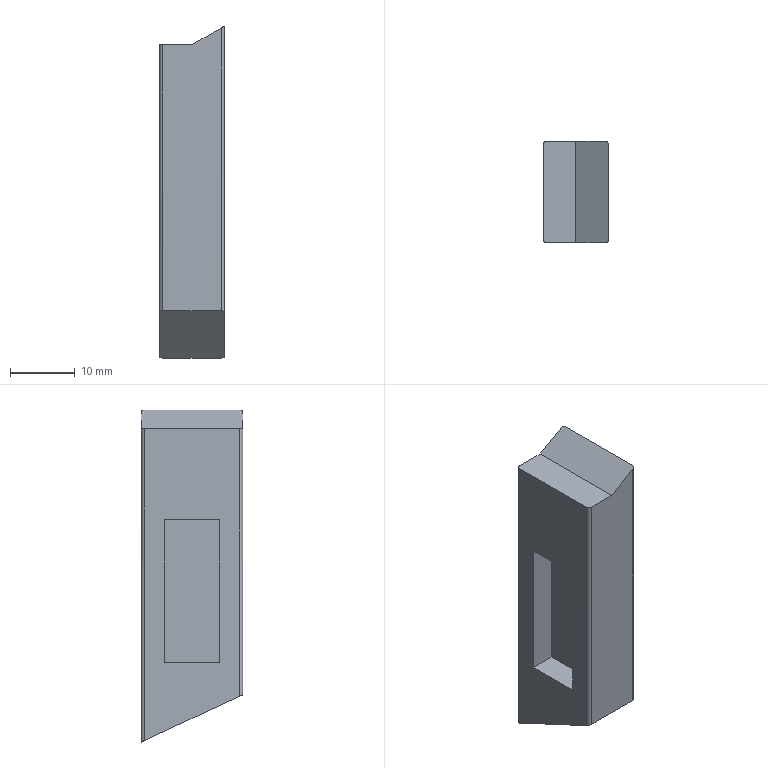Part | STEP file | luoi ga co logo | 1 solid | 16 faces | box 10 x 15.6 x 51.124 mm | volume 6311 mm3 | plane 12 | cylinder 4 | commonest cylinder face diameters 1 x4
STEP:
#1=CARTESIAN_POINT('',(0.,0.,0.));
#2=DIRECTION('',(0.,0.,1.));
#3=DIRECTION('',(1.,0.,0.));
#4=AXIS2_PLACEMENT_3D('',#1,#2,#3);
#5=CARTESIAN_POINT('',(10.,15.1,60.));
#6=VERTEX_POINT('',#5);
#7=CARTESIAN_POINT('',(10.,0.5,60.));
#8=VERTEX_POINT('',#7);
#9=CARTESIAN_POINT('',(10.,15.1,60.));
#10=DIRECTION('',(0.,-1.,0.));
#11=VECTOR('',#10,1.);
#12=LINE('',#9,#11);
#13=CARTESIAN_POINT('',(10.,15.1,0.));
#14=DIRECTION('',(1.,0.,0.));
#15=DIRECTION('',(0.,0.,-1.));
#16=AXIS2_PLACEMENT_3D('',#13,#14,#15);
#17=PLANE('',#16);
#18=CARTESIAN_POINT('',(-60.,0.));
#19=DIRECTION('',(0.,-1.));
#20=VECTOR('',#19,1.);
#21=LINE('',#18,#20);
#22=(GEOMETRIC_REPRESENTATION_CONTEXT(2)PARAMETRIC_REPRESENTATION_CONTEXT()REPRESENTATION_CONTEXT('',''));
#23=DEFINITIONAL_REPRESENTATION('',(#21),#22);
#24=PCURVE('',#17,#23);
#25=CARTESIAN_POINT('',(4.977,0.,57.1));
#26=DIRECTION('',(0.5,0.,-0.866));
#27=DIRECTION('',(-0.866,0.,-0.5));
#28=AXIS2_PLACEMENT_3D('',#25,#26,#27);
#29=PLANE('',#28);
#30=CARTESIAN_POINT('',(-5.8,15.1));
#31=DIRECTION('',(0.,-1.));
#32=VECTOR('',#31,1.);
#33=LINE('',#30,#32);
#34=(GEOMETRIC_REPRESENTATION_CONTEXT(2)PARAMETRIC_REPRESENTATION_CONTEXT()REPRESENTATION_CONTEXT('',''));
#35=DEFINITIONAL_REPRESENTATION('',(#33),#34);
#36=PCURVE('',#29,#35);
#37=SURFACE_CURVE('',#12,(#24,#36),.PCURVE_S1.);
#38=EDGE_CURVE('',#6,#8,#37,.T.);
#39=ORIENTED_EDGE('',*,*,#38,.T.);
#40=CARTESIAN_POINT('',(10.,0.5,15.917));
#41=VERTEX_POINT('',#40);
#42=CARTESIAN_POINT('',(10.,0.5,0.));
#43=DIRECTION('',(0.,0.,-1.));
#44=VECTOR('',#43,1.);
#45=LINE('',#42,#44);
#46=CARTESIAN_POINT('',(0.,-14.6));
#47=DIRECTION('',(1.,0.));
#48=VECTOR('',#47,1.);
#49=LINE('',#46,#48);
#50=(GEOMETRIC_REPRESENTATION_CONTEXT(2)PARAMETRIC_REPRESENTATION_CONTEXT()REPRESENTATION_CONTEXT('',''));
#51=DEFINITIONAL_REPRESENTATION('',(#49),#50);
#52=PCURVE('',#17,#51);
#53=CARTESIAN_POINT('',(9.5,0.5,0.));
#54=DIRECTION('',(0.,0.,1.));
#55=DIRECTION('',(1.,0.,0.));
#56=AXIS2_PLACEMENT_3D('',#53,#54,#55);
#57=CYLINDRICAL_SURFACE('',#56,0.5);
#58=CARTESIAN_POINT('',(6.283,0.));
#59=DIRECTION('',(0.,-1.));
#60=VECTOR('',#59,1.);
#61=LINE('',#58,#60);
#62=(GEOMETRIC_REPRESENTATION_CONTEXT(2)PARAMETRIC_REPRESENTATION_CONTEXT()REPRESENTATION_CONTEXT('',''));
#63=DEFINITIONAL_REPRESENTATION('',(#61),#62);
#64=PCURVE('',#57,#63);
#65=SURFACE_CURVE('',#45,(#52,#64),.PCURVE_S1.);
#66=EDGE_CURVE('',#8,#41,#65,.T.);
#67=ORIENTED_EDGE('',*,*,#66,.T.);
#68=CARTESIAN_POINT('',(10.,15.1,9.109));
#69=VERTEX_POINT('',#68);
#70=CARTESIAN_POINT('',(10.,0.5,15.917));
#71=DIRECTION('',(0.,0.9063,-0.4226));
#72=VECTOR('',#71,1.);
#73=LINE('',#70,#72);
#74=CARTESIAN_POINT('',(-15.917,-14.6));
#75=DIRECTION('',(0.4226,0.9063));
#76=VECTOR('',#75,1.);
#77=LINE('',#74,#76);
#78=(GEOMETRIC_REPRESENTATION_CONTEXT(2)PARAMETRIC_REPRESENTATION_CONTEXT()REPRESENTATION_CONTEXT('',''));
#79=DEFINITIONAL_REPRESENTATION('',(#77),#78);
#80=PCURVE('',#17,#79);
#81=CARTESIAN_POINT('',(0.,0.,16.15));
#82=DIRECTION('',(0.,0.4226,0.9063));
#83=DIRECTION('',(0.,-0.9063,0.4226));
#84=AXIS2_PLACEMENT_3D('',#81,#82,#83);
#85=PLANE('',#84);
#86=CARTESIAN_POINT('',(-0.5517,10.));
#87=DIRECTION('',(-1.,0.));
#88=VECTOR('',#87,1.);
#89=LINE('',#86,#88);
#90=(GEOMETRIC_REPRESENTATION_CONTEXT(2)PARAMETRIC_REPRESENTATION_CONTEXT()REPRESENTATION_CONTEXT('',''));
#91=DEFINITIONAL_REPRESENTATION('',(#89),#90);
#92=PCURVE('',#85,#91);
#93=SURFACE_CURVE('',#73,(#80,#92),.PCURVE_S1.);
#94=EDGE_CURVE('',#41,#69,#93,.T.);
#95=ORIENTED_EDGE('',*,*,#94,.T.);
#96=CARTESIAN_POINT('',(10.,15.1,0.));
#97=DIRECTION('',(0.,0.,1.));
#98=VECTOR('',#97,1.);
#99=LINE('',#96,#98);
#100=CARTESIAN_POINT('',(0.,0.));
#101=DIRECTION('',(-1.,0.));
#102=VECTOR('',#101,1.);
#103=LINE('',#100,#102);
#104=(GEOMETRIC_REPRESENTATION_CONTEXT(2)PARAMETRIC_REPRESENTATION_CONTEXT()REPRESENTATION_CONTEXT('',''));
#105=DEFINITIONAL_REPRESENTATION('',(#103),#104);
#106=PCURVE('',#17,#105);
#107=CARTESIAN_POINT('',(9.5,15.1,0.));
#108=DIRECTION('',(0.,0.,1.));
#109=DIRECTION('',(1.,0.,0.));
#110=AXIS2_PLACEMENT_3D('',#107,#108,#109);
#111=CYLINDRICAL_SURFACE('',#110,0.5);
#112=CARTESIAN_POINT('',(0.,0.));
#113=DIRECTION('',(0.,1.));
#114=VECTOR('',#113,1.);
#115=LINE('',#112,#114);
#116=(GEOMETRIC_REPRESENTATION_CONTEXT(2)PARAMETRIC_REPRESENTATION_CONTEXT()REPRESENTATION_CONTEXT('',''));
#117=DEFINITIONAL_REPRESENTATION('',(#115),#116);
#118=PCURVE('',#111,#117);
#119=SURFACE_CURVE('',#99,(#106,#118),.PCURVE_S1.);
#120=EDGE_CURVE('',#69,#6,#119,.T.);
#121=ORIENTED_EDGE('',*,*,#120,.T.);
#122=EDGE_LOOP('',(#39,#67,#95,#121));
#123=FACE_BOUND('',#122,.T.);
#124=ADVANCED_FACE('',(#123),#17,.T.);
#125=CARTESIAN_POINT('',(9.5,0.,59.711));
#126=VERTEX_POINT('',#125);
#127=CARTESIAN_POINT('',(10.,0.5,60.));
#128=CARTESIAN_POINT('',(10.,0.2071,60.));
#129=CARTESIAN_POINT('',(9.793,0.,59.88));
#130=CARTESIAN_POINT('',(9.5,0.,59.711));
#131=(BOUNDED_CURVE()B_SPLINE_CURVE(3,(#127,#128,#129,#130),.UNSPECIFIED.,.F.,.F.)B_SPLINE_CURVE_WITH_KNOTS((4,4),(0.,1.571),.PIECEWISE_BEZIER_KNOTS.)CURVE()GEOMETRIC_REPRESENTATION_ITEM()RATIONAL_B_SPLINE_CURVE((1.,0.8047,0.8047,1.))REPRESENTATION_ITEM(''));
#132=CARTESIAN_POINT('',(6.283,60.));
#133=CARTESIAN_POINT('',(6.262,60.));
#134=CARTESIAN_POINT('',(6.218,60.));
#135=CARTESIAN_POINT('',(6.152,59.998));
#136=CARTESIAN_POINT('',(6.083,59.994));
#137=CARTESIAN_POINT('',(6.013,59.99));
#138=CARTESIAN_POINT('',(5.942,59.984));
#139=CARTESIAN_POINT('',(5.87,59.976));
#140=CARTESIAN_POINT('',(5.797,59.967));
#141=CARTESIAN_POINT('',(5.723,59.956));
#142=CARTESIAN_POINT('',(5.648,59.944));
#143=CARTESIAN_POINT('',(5.573,59.93));
#144=CARTESIAN_POINT('',(5.498,59.916));
#145=CARTESIAN_POINT('',(5.422,59.9));
#146=CARTESIAN_POINT('',(5.347,59.883));
#147=CARTESIAN_POINT('',(5.273,59.865));
#148=CARTESIAN_POINT('',(5.199,59.846));
#149=CARTESIAN_POINT('',(5.125,59.827));
#150=CARTESIAN_POINT('',(5.053,59.808));
#151=CARTESIAN_POINT('',(4.982,59.788));
#152=CARTESIAN_POINT('',(4.912,59.769));
#153=CARTESIAN_POINT('',(4.844,59.749));
#154=CARTESIAN_POINT('',(4.777,59.73));
#155=CARTESIAN_POINT('',(4.734,59.718));
#156=CARTESIAN_POINT('',(4.712,59.711));
#157=B_SPLINE_CURVE_WITH_KNOTS('',3,(#132,#133,#134,#135,#136,#137,#138,#139,#140,#141,#142,#143,#144,#145,#146,#147,#148,#149,#150,#151,#152,#153,#154,#155,#156),.UNSPECIFIED.,.F.,.F.,(4,1,1,1,1,1,1,1,1,1,1,1,1,1,1,1,1,1,1,1,1,1,4),(0.,0.0714,0.1428,0.2142,0.2856,0.357,0.4284,0.4998,0.5712,0.6426,0.714,0.7854,0.8568,0.9282,0.9996,1.071,1.142,1.214,1.285,1.357,1.428,1.499,1.571),.QUASI_UNIFORM_KNOTS.);
#158=(GEOMETRIC_REPRESENTATION_CONTEXT(2)PARAMETRIC_REPRESENTATION_CONTEXT()REPRESENTATION_CONTEXT('',''));
#159=DEFINITIONAL_REPRESENTATION('',(#157),#158);
#160=PCURVE('',#57,#159);
#161=CARTESIAN_POINT('',(-5.8,0.5));
#162=CARTESIAN_POINT('',(-5.8,0.2071));
#163=CARTESIAN_POINT('',(-5.561,0.));
#164=CARTESIAN_POINT('',(-5.223,0.));
#165=(BOUNDED_CURVE()B_SPLINE_CURVE(3,(#161,#162,#163,#164),.UNSPECIFIED.,.F.,.F.)B_SPLINE_CURVE_WITH_KNOTS((4,4),(0.,1.571),.PIECEWISE_BEZIER_KNOTS.)CURVE()GEOMETRIC_REPRESENTATION_ITEM()RATIONAL_B_SPLINE_CURVE((1.,0.8047,0.8047,1.))REPRESENTATION_ITEM(''));
#166=(GEOMETRIC_REPRESENTATION_CONTEXT(2)PARAMETRIC_REPRESENTATION_CONTEXT()REPRESENTATION_CONTEXT('',''));
#167=DEFINITIONAL_REPRESENTATION('',(#165),#166);
#168=PCURVE('',#29,#167);
#169=SURFACE_CURVE('',#131,(#160,#168),.PCURVE_S1.);
#170=EDGE_CURVE('',#8,#126,#169,.T.);
#171=ORIENTED_EDGE('',*,*,#170,.T.);
#172=CARTESIAN_POINT('',(9.5,0.,16.15));
#173=VERTEX_POINT('',#172);
#174=CARTESIAN_POINT('',(9.5,0.,0.));
#175=DIRECTION('',(0.,0.,-1.));
#176=VECTOR('',#175,1.);
#177=LINE('',#174,#176);
#178=CARTESIAN_POINT('',(4.712,0.));
#179=DIRECTION('',(0.,-1.));
#180=VECTOR('',#179,1.);
#181=LINE('',#178,#180);
#182=(GEOMETRIC_REPRESENTATION_CONTEXT(2)PARAMETRIC_REPRESENTATION_CONTEXT()REPRESENTATION_CONTEXT('',''));
#183=DEFINITIONAL_REPRESENTATION('',(#181),#182);
#184=PCURVE('',#57,#183);
#185=CARTESIAN_POINT('',(9.5,0.,0.));
#186=DIRECTION('',(0.,-1.,0.));
#187=DIRECTION('',(0.,0.,-1.));
#188=AXIS2_PLACEMENT_3D('',#185,#186,#187);
#189=PLANE('',#188);
#190=CARTESIAN_POINT('',(0.,0.));
#191=DIRECTION('',(1.,0.));
#192=VECTOR('',#191,1.);
#193=LINE('',#190,#192);
#194=(GEOMETRIC_REPRESENTATION_CONTEXT(2)PARAMETRIC_REPRESENTATION_CONTEXT()REPRESENTATION_CONTEXT('',''));
#195=DEFINITIONAL_REPRESENTATION('',(#193),#194);
#196=PCURVE('',#189,#195);
#197=SURFACE_CURVE('',#177,(#184,#196),.PCURVE_S1.);
#198=EDGE_CURVE('',#126,#173,#197,.T.);
#199=ORIENTED_EDGE('',*,*,#198,.T.);
#200=CARTESIAN_POINT('',(9.5,0.,16.15));
#201=CARTESIAN_POINT('',(9.793,0.,16.15));
#202=CARTESIAN_POINT('',(10.,0.2071,16.054));
#203=CARTESIAN_POINT('',(10.,0.5,15.917));
#204=(BOUNDED_CURVE()B_SPLINE_CURVE(3,(#200,#201,#202,#203),.UNSPECIFIED.,.F.,.F.)B_SPLINE_CURVE_WITH_KNOTS((4,4),(0.,1.571),.PIECEWISE_BEZIER_KNOTS.)CURVE()GEOMETRIC_REPRESENTATION_ITEM()RATIONAL_B_SPLINE_CURVE((1.,0.8047,0.8047,1.))REPRESENTATION_ITEM(''));
#205=CARTESIAN_POINT('',(4.712,16.15));
#206=CARTESIAN_POINT('',(4.734,16.15));
#207=CARTESIAN_POINT('',(4.777,16.15));
#208=CARTESIAN_POINT('',(4.844,16.149));
#209=CARTESIAN_POINT('',(4.912,16.146));
#210=CARTESIAN_POINT('',(4.982,16.142));
#211=CARTESIAN_POINT('',(5.053,16.137));
#212=CARTESIAN_POINT('',(5.125,16.131));
#213=CARTESIAN_POINT('',(5.199,16.124));
#214=CARTESIAN_POINT('',(5.273,16.115));
#215=CARTESIAN_POINT('',(5.347,16.105));
#216=CARTESIAN_POINT('',(5.422,16.094));
#217=CARTESIAN_POINT('',(5.498,16.082));
#218=CARTESIAN_POINT('',(5.573,16.069));
#219=CARTESIAN_POINT('',(5.648,16.056));
#220=CARTESIAN_POINT('',(5.723,16.041));
#221=CARTESIAN_POINT('',(5.797,16.026));
#222=CARTESIAN_POINT('',(5.87,16.011));
#223=CARTESIAN_POINT('',(5.942,15.995));
#224=CARTESIAN_POINT('',(6.013,15.979));
#225=CARTESIAN_POINT('',(6.083,15.964));
#226=CARTESIAN_POINT('',(6.152,15.948));
#227=CARTESIAN_POINT('',(6.218,15.932));
#228=CARTESIAN_POINT('',(6.262,15.922));
#229=CARTESIAN_POINT('',(6.283,15.917));
#230=B_SPLINE_CURVE_WITH_KNOTS('',3,(#205,#206,#207,#208,#209,#210,#211,#212,#213,#214,#215,#216,#217,#218,#219,#220,#221,#222,#223,#224,#225,#226,#227,#228,#229),.UNSPECIFIED.,.F.,.F.,(4,1,1,1,1,1,1,1,1,1,1,1,1,1,1,1,1,1,1,1,1,1,4),(0.,0.0714,0.1428,0.2142,0.2856,0.357,0.4284,0.4998,0.5712,0.6426,0.714,0.7854,0.8568,0.9282,0.9996,1.071,1.142,1.214,1.285,1.357,1.428,1.499,1.571),.QUASI_UNIFORM_KNOTS.);
#231=(GEOMETRIC_REPRESENTATION_CONTEXT(2)PARAMETRIC_REPRESENTATION_CONTEXT()REPRESENTATION_CONTEXT('',''));
#232=DEFINITIONAL_REPRESENTATION('',(#230),#231);
#233=PCURVE('',#57,#232);
#234=CARTESIAN_POINT('',(0.,9.5));
#235=CARTESIAN_POINT('',(0.,9.793));
#236=CARTESIAN_POINT('',(-0.2285,10.));
#237=CARTESIAN_POINT('',(-0.5517,10.));
#238=(BOUNDED_CURVE()B_SPLINE_CURVE(3,(#234,#235,#236,#237),.UNSPECIFIED.,.F.,.F.)B_SPLINE_CURVE_WITH_KNOTS((4,4),(0.,1.571),.PIECEWISE_BEZIER_KNOTS.)CURVE()GEOMETRIC_REPRESENTATION_ITEM()RATIONAL_B_SPLINE_CURVE((1.,0.8047,0.8047,1.))REPRESENTATION_ITEM(''));
#239=(GEOMETRIC_REPRESENTATION_CONTEXT(2)PARAMETRIC_REPRESENTATION_CONTEXT()REPRESENTATION_CONTEXT('',''));
#240=DEFINITIONAL_REPRESENTATION('',(#238),#239);
#241=PCURVE('',#85,#240);
#242=SURFACE_CURVE('',#204,(#233,#241),.PCURVE_S1.);
#243=EDGE_CURVE('',#173,#41,#242,.T.);
#244=ORIENTED_EDGE('',*,*,#243,.T.);
#245=ORIENTED_EDGE('',*,*,#66,.F.);
#246=EDGE_LOOP('',(#171,#199,#244,#245));
#247=FACE_BOUND('',#246,.T.);
#248=ADVANCED_FACE('',(#247),#57,.T.);
#249=ORIENTED_EDGE('',*,*,#38,.F.);
#250=CARTESIAN_POINT('',(9.5,15.6,59.711));
#251=VERTEX_POINT('',#250);
#252=CARTESIAN_POINT('',(9.5,15.6,59.711));
#253=CARTESIAN_POINT('',(9.793,15.6,59.88));
#254=CARTESIAN_POINT('',(10.,15.393,60.));
#255=CARTESIAN_POINT('',(10.,15.1,60.));
#256=(BOUNDED_CURVE()B_SPLINE_CURVE(3,(#252,#253,#254,#255),.UNSPECIFIED.,.F.,.F.)B_SPLINE_CURVE_WITH_KNOTS((4,4),(4.712,6.283),.PIECEWISE_BEZIER_KNOTS.)CURVE()GEOMETRIC_REPRESENTATION_ITEM()RATIONAL_B_SPLINE_CURVE((1.,0.8047,0.8047,1.))REPRESENTATION_ITEM(''));
#257=CARTESIAN_POINT('',(-5.223,15.6));
#258=CARTESIAN_POINT('',(-5.561,15.6));
#259=CARTESIAN_POINT('',(-5.8,15.393));
#260=CARTESIAN_POINT('',(-5.8,15.1));
#261=(BOUNDED_CURVE()B_SPLINE_CURVE(3,(#257,#258,#259,#260),.UNSPECIFIED.,.F.,.F.)B_SPLINE_CURVE_WITH_KNOTS((4,4),(4.712,6.283),.PIECEWISE_BEZIER_KNOTS.)CURVE()GEOMETRIC_REPRESENTATION_ITEM()RATIONAL_B_SPLINE_CURVE((1.,0.8047,0.8047,1.))REPRESENTATION_ITEM(''));
#262=(GEOMETRIC_REPRESENTATION_CONTEXT(2)PARAMETRIC_REPRESENTATION_CONTEXT()REPRESENTATION_CONTEXT('',''));
#263=DEFINITIONAL_REPRESENTATION('',(#261),#262);
#264=PCURVE('',#29,#263);
#265=CARTESIAN_POINT('',(1.571,59.711));
#266=CARTESIAN_POINT('',(1.549,59.718));
#267=CARTESIAN_POINT('',(1.506,59.73));
#268=CARTESIAN_POINT('',(1.439,59.749));
#269=CARTESIAN_POINT('',(1.371,59.769));
#270=CARTESIAN_POINT('',(1.301,59.788));
#271=CARTESIAN_POINT('',(1.23,59.808));
#272=CARTESIAN_POINT('',(1.158,59.827));
#273=CARTESIAN_POINT('',(1.085,59.846));
#274=CARTESIAN_POINT('',(1.01,59.865));
#275=CARTESIAN_POINT('',(0.9358,59.883));
#276=CARTESIAN_POINT('',(0.8607,59.9));
#277=CARTESIAN_POINT('',(0.7854,59.916));
#278=CARTESIAN_POINT('',(0.7101,59.93));
#279=CARTESIAN_POINT('',(0.635,59.944));
#280=CARTESIAN_POINT('',(0.5603,59.956));
#281=CARTESIAN_POINT('',(0.4863,59.967));
#282=CARTESIAN_POINT('',(0.413,59.976));
#283=CARTESIAN_POINT('',(0.3408,59.984));
#284=CARTESIAN_POINT('',(0.2697,59.99));
#285=CARTESIAN_POINT('',(0.2,59.994));
#286=CARTESIAN_POINT('',(0.1316,59.998));
#287=CARTESIAN_POINT('',(0.06485,60.));
#288=CARTESIAN_POINT('',(0.02143,60.));
#289=CARTESIAN_POINT('',(0.,60.));
#290=B_SPLINE_CURVE_WITH_KNOTS('',3,(#265,#266,#267,#268,#269,#270,#271,#272,#273,#274,#275,#276,#277,#278,#279,#280,#281,#282,#283,#284,#285,#286,#287,#288,#289),.UNSPECIFIED.,.F.,.F.,(4,1,1,1,1,1,1,1,1,1,1,1,1,1,1,1,1,1,1,1,1,1,4),(4.712,4.784,4.855,4.927,4.998,5.069,5.141,5.212,5.284,5.355,5.426,5.498,5.569,5.641,5.712,5.783,5.855,5.926,5.998,6.069,6.14,6.212,6.283),.QUASI_UNIFORM_KNOTS.);
#291=(GEOMETRIC_REPRESENTATION_CONTEXT(2)PARAMETRIC_REPRESENTATION_CONTEXT()REPRESENTATION_CONTEXT('',''));
#292=DEFINITIONAL_REPRESENTATION('',(#290),#291);
#293=PCURVE('',#111,#292);
#294=SURFACE_CURVE('',#256,(#264,#293),.PCURVE_S1.);
#295=EDGE_CURVE('',#251,#6,#294,.T.);
#296=ORIENTED_EDGE('',*,*,#295,.F.);
#297=CARTESIAN_POINT('',(4.977,15.6,57.1));
#298=VERTEX_POINT('',#297);
#299=CARTESIAN_POINT('',(4.977,15.6,57.1));
#300=DIRECTION('',(0.866,0.,0.5));
#301=VECTOR('',#300,1.);
#302=LINE('',#299,#301);
#303=CARTESIAN_POINT('',(0.,15.6));
#304=DIRECTION('',(-1.,0.));
#305=VECTOR('',#304,1.);
#306=LINE('',#303,#305);
#307=(GEOMETRIC_REPRESENTATION_CONTEXT(2)PARAMETRIC_REPRESENTATION_CONTEXT()REPRESENTATION_CONTEXT('',''));
#308=DEFINITIONAL_REPRESENTATION('',(#306),#307);
#309=PCURVE('',#29,#308);
#310=CARTESIAN_POINT('',(0.5,15.6,0.));
#311=DIRECTION('',(0.,1.,0.));
#312=DIRECTION('',(0.,0.,1.));
#313=AXIS2_PLACEMENT_3D('',#310,#311,#312);
#314=PLANE('',#313);
#315=CARTESIAN_POINT('',(57.1,4.477));
#316=DIRECTION('',(0.5,0.866));
#317=VECTOR('',#316,1.);
#318=LINE('',#315,#317);
#319=(GEOMETRIC_REPRESENTATION_CONTEXT(2)PARAMETRIC_REPRESENTATION_CONTEXT()REPRESENTATION_CONTEXT('',''));
#320=DEFINITIONAL_REPRESENTATION('',(#318),#319);
#321=PCURVE('',#314,#320);
#322=SURFACE_CURVE('',#302,(#309,#321),.PCURVE_S1.);
#323=EDGE_CURVE('',#298,#251,#322,.T.);
#324=ORIENTED_EDGE('',*,*,#323,.F.);
#325=CARTESIAN_POINT('',(4.977,0.,57.1));
#326=VERTEX_POINT('',#325);
#327=CARTESIAN_POINT('',(4.977,0.,57.1));
#328=DIRECTION('',(0.,1.,0.));
#329=VECTOR('',#328,1.);
#330=LINE('',#327,#329);
#331=CARTESIAN_POINT('',(0.,0.));
#332=DIRECTION('',(0.,1.));
#333=VECTOR('',#332,1.);
#334=LINE('',#331,#333);
#335=(GEOMETRIC_REPRESENTATION_CONTEXT(2)PARAMETRIC_REPRESENTATION_CONTEXT()REPRESENTATION_CONTEXT('',''));
#336=DEFINITIONAL_REPRESENTATION('',(#334),#335);
#337=PCURVE('',#29,#336);
#338=CARTESIAN_POINT('',(-5.,0.,57.1));
#339=DIRECTION('',(0.,0.,-1.));
#340=DIRECTION('',(-1.,0.,0.));
#341=AXIS2_PLACEMENT_3D('',#338,#339,#340);
#342=PLANE('',#341);
#343=CARTESIAN_POINT('',(-9.977,0.));
#344=DIRECTION('',(0.,1.));
#345=VECTOR('',#344,1.);
#346=LINE('',#343,#345);
#347=(GEOMETRIC_REPRESENTATION_CONTEXT(2)PARAMETRIC_REPRESENTATION_CONTEXT()REPRESENTATION_CONTEXT('',''));
#348=DEFINITIONAL_REPRESENTATION('',(#346),#347);
#349=PCURVE('',#342,#348);
#350=SURFACE_CURVE('',#330,(#337,#349),.PCURVE_S1.);
#351=EDGE_CURVE('',#326,#298,#350,.T.);
#352=ORIENTED_EDGE('',*,*,#351,.F.);
#353=CARTESIAN_POINT('',(4.977,0.,57.1));
#354=DIRECTION('',(-0.866,0.,-0.5));
#355=VECTOR('',#354,1.);
#356=LINE('',#353,#355);
#357=CARTESIAN_POINT('',(0.,0.));
#358=DIRECTION('',(1.,0.));
#359=VECTOR('',#358,1.);
#360=LINE('',#357,#359);
#361=(GEOMETRIC_REPRESENTATION_CONTEXT(2)PARAMETRIC_REPRESENTATION_CONTEXT()REPRESENTATION_CONTEXT('',''));
#362=DEFINITIONAL_REPRESENTATION('',(#360),#361);
#363=PCURVE('',#29,#362);
#364=CARTESIAN_POINT('',(-57.1,-4.523));
#365=DIRECTION('',(0.5,-0.866));
#366=VECTOR('',#365,1.);
#367=LINE('',#364,#366);
#368=(GEOMETRIC_REPRESENTATION_CONTEXT(2)PARAMETRIC_REPRESENTATION_CONTEXT()REPRESENTATION_CONTEXT('',''));
#369=DEFINITIONAL_REPRESENTATION('',(#367),#368);
#370=PCURVE('',#189,#369);
#371=SURFACE_CURVE('',#356,(#363,#370),.PCURVE_S1.);
#372=EDGE_CURVE('',#126,#326,#371,.T.);
#373=ORIENTED_EDGE('',*,*,#372,.F.);
#374=ORIENTED_EDGE('',*,*,#170,.F.);
#375=EDGE_LOOP('',(#249,#296,#324,#352,#373,#374));
#376=FACE_BOUND('',#375,.T.);
#377=ADVANCED_FACE('',(#376),#29,.F.);
#378=ORIENTED_EDGE('',*,*,#295,.T.);
#379=ORIENTED_EDGE('',*,*,#120,.F.);
#380=CARTESIAN_POINT('',(9.5,15.6,8.876));
#381=VERTEX_POINT('',#380);
#382=CARTESIAN_POINT('',(10.,15.1,9.109));
#383=CARTESIAN_POINT('',(10.,15.393,8.973));
#384=CARTESIAN_POINT('',(9.793,15.6,8.876));
#385=CARTESIAN_POINT('',(9.5,15.6,8.876));
#386=(BOUNDED_CURVE()B_SPLINE_CURVE(3,(#382,#383,#384,#385),.UNSPECIFIED.,.F.,.F.)B_SPLINE_CURVE_WITH_KNOTS((4,4),(1.571,3.142),.PIECEWISE_BEZIER_KNOTS.)CURVE()GEOMETRIC_REPRESENTATION_ITEM()RATIONAL_B_SPLINE_CURVE((1.,0.8047,0.8047,1.))REPRESENTATION_ITEM(''));
#387=CARTESIAN_POINT('',(0.,9.109));
#388=CARTESIAN_POINT('',(0.02143,9.104));
#389=CARTESIAN_POINT('',(0.06485,9.094));
#390=CARTESIAN_POINT('',(0.1316,9.079));
#391=CARTESIAN_POINT('',(0.2,9.063));
#392=CARTESIAN_POINT('',(0.2697,9.047));
#393=CARTESIAN_POINT('',(0.3408,9.031));
#394=CARTESIAN_POINT('',(0.413,9.015));
#395=CARTESIAN_POINT('',(0.4863,9.));
#396=CARTESIAN_POINT('',(0.5603,8.985));
#397=CARTESIAN_POINT('',(0.635,8.971));
#398=CARTESIAN_POINT('',(0.7101,8.957));
#399=CARTESIAN_POINT('',(0.7854,8.944));
#400=CARTESIAN_POINT('',(0.8607,8.932));
#401=CARTESIAN_POINT('',(0.9358,8.921));
#402=CARTESIAN_POINT('',(1.01,8.911));
#403=CARTESIAN_POINT('',(1.085,8.903));
#404=CARTESIAN_POINT('',(1.158,8.895));
#405=CARTESIAN_POINT('',(1.23,8.889));
#406=CARTESIAN_POINT('',(1.301,8.884));
#407=CARTESIAN_POINT('',(1.371,8.88));
#408=CARTESIAN_POINT('',(1.439,8.878));
#409=CARTESIAN_POINT('',(1.506,8.876));
#410=CARTESIAN_POINT('',(1.549,8.876));
#411=CARTESIAN_POINT('',(1.571,8.876));
#412=B_SPLINE_CURVE_WITH_KNOTS('',3,(#387,#388,#389,#390,#391,#392,#393,#394,#395,#396,#397,#398,#399,#400,#401,#402,#403,#404,#405,#406,#407,#408,#409,#410,#411),.UNSPECIFIED.,.F.,.F.,(4,1,1,1,1,1,1,1,1,1,1,1,1,1,1,1,1,1,1,1,1,1,4),(1.571,1.642,1.714,1.785,1.856,1.928,1.999,2.071,2.142,2.213,2.285,2.356,2.428,2.499,2.57,2.642,2.713,2.785,2.856,2.927,2.999,3.07,3.142),.QUASI_UNIFORM_KNOTS.);
#413=(GEOMETRIC_REPRESENTATION_CONTEXT(2)PARAMETRIC_REPRESENTATION_CONTEXT()REPRESENTATION_CONTEXT('',''));
#414=DEFINITIONAL_REPRESENTATION('',(#412),#413);
#415=PCURVE('',#111,#414);
#416=CARTESIAN_POINT('',(-16.661,10.));
#417=CARTESIAN_POINT('',(-16.984,10.));
#418=CARTESIAN_POINT('',(-17.213,9.793));
#419=CARTESIAN_POINT('',(-17.213,9.5));
#420=(BOUNDED_CURVE()B_SPLINE_CURVE(3,(#416,#417,#418,#419),.UNSPECIFIED.,.F.,.F.)B_SPLINE_CURVE_WITH_KNOTS((4,4),(1.571,3.142),.PIECEWISE_BEZIER_KNOTS.)CURVE()GEOMETRIC_REPRESENTATION_ITEM()RATIONAL_B_SPLINE_CURVE((1.,0.8047,0.8047,1.))REPRESENTATION_ITEM(''));
#421=(GEOMETRIC_REPRESENTATION_CONTEXT(2)PARAMETRIC_REPRESENTATION_CONTEXT()REPRESENTATION_CONTEXT('',''));
#422=DEFINITIONAL_REPRESENTATION('',(#420),#421);
#423=PCURVE('',#85,#422);
#424=SURFACE_CURVE('',#386,(#415,#423),.PCURVE_S1.);
#425=EDGE_CURVE('',#69,#381,#424,.T.);
#426=ORIENTED_EDGE('',*,*,#425,.T.);
#427=CARTESIAN_POINT('',(9.5,15.6,0.));
#428=DIRECTION('',(0.,0.,1.));
#429=VECTOR('',#428,1.);
#430=LINE('',#427,#429);
#431=CARTESIAN_POINT('',(1.571,0.));
#432=DIRECTION('',(0.,1.));
#433=VECTOR('',#432,1.);
#434=LINE('',#431,#433);
#435=(GEOMETRIC_REPRESENTATION_CONTEXT(2)PARAMETRIC_REPRESENTATION_CONTEXT()REPRESENTATION_CONTEXT('',''));
#436=DEFINITIONAL_REPRESENTATION('',(#434),#435);
#437=PCURVE('',#111,#436);
#438=CARTESIAN_POINT('',(0.,9.));
#439=DIRECTION('',(1.,0.));
#440=VECTOR('',#439,1.);
#441=LINE('',#438,#440);
#442=(GEOMETRIC_REPRESENTATION_CONTEXT(2)PARAMETRIC_REPRESENTATION_CONTEXT()REPRESENTATION_CONTEXT('',''));
#443=DEFINITIONAL_REPRESENTATION('',(#441),#442);
#444=PCURVE('',#314,#443);
#445=SURFACE_CURVE('',#430,(#437,#444),.PCURVE_S1.);
#446=EDGE_CURVE('',#381,#251,#445,.T.);
#447=ORIENTED_EDGE('',*,*,#446,.T.);
#448=EDGE_LOOP('',(#378,#379,#426,#447));
#449=FACE_BOUND('',#448,.T.);
#450=ADVANCED_FACE('',(#449),#111,.T.);
#451=CARTESIAN_POINT('',(0.5,15.6,8.876));
#452=VERTEX_POINT('',#451);
#453=CARTESIAN_POINT('',(0.,15.6,8.876));
#454=DIRECTION('',(-1.,0.,0.));
#455=VECTOR('',#454,1.);
#456=LINE('',#453,#455);
#457=CARTESIAN_POINT('',(-17.213,0.));
#458=DIRECTION('',(0.,-1.));
#459=VECTOR('',#458,1.);
#460=LINE('',#457,#459);
#461=(GEOMETRIC_REPRESENTATION_CONTEXT(2)PARAMETRIC_REPRESENTATION_CONTEXT()REPRESENTATION_CONTEXT('',''));
#462=DEFINITIONAL_REPRESENTATION('',(#460),#461);
#463=PCURVE('',#85,#462);
#464=CARTESIAN_POINT('',(8.876,-0.5));
#465=DIRECTION('',(0.,-1.));
#466=VECTOR('',#465,1.);
#467=LINE('',#464,#466);
#468=(GEOMETRIC_REPRESENTATION_CONTEXT(2)PARAMETRIC_REPRESENTATION_CONTEXT()REPRESENTATION_CONTEXT('',''));
#469=DEFINITIONAL_REPRESENTATION('',(#467),#468);
#470=PCURVE('',#314,#469);
#471=SURFACE_CURVE('',#456,(#463,#470),.PCURVE_S1.);
#472=EDGE_CURVE('',#381,#452,#471,.T.);
#473=ORIENTED_EDGE('',*,*,#472,.F.);
#474=ORIENTED_EDGE('',*,*,#425,.F.);
#475=ORIENTED_EDGE('',*,*,#94,.F.);
#476=ORIENTED_EDGE('',*,*,#243,.F.);
#477=CARTESIAN_POINT('',(0.5,0.,16.15));
#478=VERTEX_POINT('',#477);
#479=CARTESIAN_POINT('',(0.,0.,16.15));
#480=DIRECTION('',(1.,0.,0.));
#481=VECTOR('',#480,1.);
#482=LINE('',#479,#481);
#483=CARTESIAN_POINT('',(0.,0.));
#484=DIRECTION('',(0.,1.));
#485=VECTOR('',#484,1.);
#486=LINE('',#483,#485);
#487=(GEOMETRIC_REPRESENTATION_CONTEXT(2)PARAMETRIC_REPRESENTATION_CONTEXT()REPRESENTATION_CONTEXT('',''));
#488=DEFINITIONAL_REPRESENTATION('',(#486),#487);
#489=PCURVE('',#85,#488);
#490=CARTESIAN_POINT('',(-16.15,-9.5));
#491=DIRECTION('',(0.,1.));
#492=VECTOR('',#491,1.);
#493=LINE('',#490,#492);
#494=(GEOMETRIC_REPRESENTATION_CONTEXT(2)PARAMETRIC_REPRESENTATION_CONTEXT()REPRESENTATION_CONTEXT('',''));
#495=DEFINITIONAL_REPRESENTATION('',(#493),#494);
#496=PCURVE('',#189,#495);
#497=SURFACE_CURVE('',#482,(#489,#496),.PCURVE_S1.);
#498=EDGE_CURVE('',#478,#173,#497,.T.);
#499=ORIENTED_EDGE('',*,*,#498,.F.);
#500=CARTESIAN_POINT('',(0.,0.5,15.917));
#501=VERTEX_POINT('',#500);
#502=CARTESIAN_POINT('',(0.,0.5,15.917));
#503=CARTESIAN_POINT('',(0.,0.2071,16.054));
#504=CARTESIAN_POINT('',(0.2071,0.,16.15));
#505=CARTESIAN_POINT('',(0.5,0.,16.15));
#506=(BOUNDED_CURVE()B_SPLINE_CURVE(3,(#502,#503,#504,#505),.UNSPECIFIED.,.F.,.F.)B_SPLINE_CURVE_WITH_KNOTS((4,4),(4.712,6.283),.PIECEWISE_BEZIER_KNOTS.)CURVE()GEOMETRIC_REPRESENTATION_ITEM()RATIONAL_B_SPLINE_CURVE((1.,0.8047,0.8047,1.))REPRESENTATION_ITEM(''));
#507=CARTESIAN_POINT('',(-0.5517,0.));
#508=CARTESIAN_POINT('',(-0.2285,0.));
#509=CARTESIAN_POINT('',(0.,0.2071));
#510=CARTESIAN_POINT('',(0.,0.5));
#511=(BOUNDED_CURVE()B_SPLINE_CURVE(3,(#507,#508,#509,#510),.UNSPECIFIED.,.F.,.F.)B_SPLINE_CURVE_WITH_KNOTS((4,4),(4.712,6.283),.PIECEWISE_BEZIER_KNOTS.)CURVE()GEOMETRIC_REPRESENTATION_ITEM()RATIONAL_B_SPLINE_CURVE((1.,0.8047,0.8047,1.))REPRESENTATION_ITEM(''));
#512=(GEOMETRIC_REPRESENTATION_CONTEXT(2)PARAMETRIC_REPRESENTATION_CONTEXT()REPRESENTATION_CONTEXT('',''));
#513=DEFINITIONAL_REPRESENTATION('',(#511),#512);
#514=PCURVE('',#85,#513);
#515=CARTESIAN_POINT('',(0.5,0.5,0.));
#516=DIRECTION('',(0.,0.,1.));
#517=DIRECTION('',(1.,0.,0.));
#518=AXIS2_PLACEMENT_3D('',#515,#516,#517);
#519=CYLINDRICAL_SURFACE('',#518,0.5);
#520=CARTESIAN_POINT('',(3.142,15.917));
#521=CARTESIAN_POINT('',(3.163,15.922));
#522=CARTESIAN_POINT('',(3.206,15.932));
#523=CARTESIAN_POINT('',(3.273,15.948));
#524=CARTESIAN_POINT('',(3.342,15.964));
#525=CARTESIAN_POINT('',(3.411,15.979));
#526=CARTESIAN_POINT('',(3.482,15.995));
#527=CARTESIAN_POINT('',(3.555,16.011));
#528=CARTESIAN_POINT('',(3.628,16.026));
#529=CARTESIAN_POINT('',(3.702,16.041));
#530=CARTESIAN_POINT('',(3.777,16.056));
#531=CARTESIAN_POINT('',(3.852,16.069));
#532=CARTESIAN_POINT('',(3.927,16.082));
#533=CARTESIAN_POINT('',(4.002,16.094));
#534=CARTESIAN_POINT('',(4.077,16.105));
#535=CARTESIAN_POINT('',(4.152,16.115));
#536=CARTESIAN_POINT('',(4.226,16.124));
#537=CARTESIAN_POINT('',(4.299,16.131));
#538=CARTESIAN_POINT('',(4.372,16.137));
#539=CARTESIAN_POINT('',(4.443,16.142));
#540=CARTESIAN_POINT('',(4.512,16.146));
#541=CARTESIAN_POINT('',(4.581,16.149));
#542=CARTESIAN_POINT('',(4.648,16.15));
#543=CARTESIAN_POINT('',(4.691,16.15));
#544=CARTESIAN_POINT('',(4.712,16.15));
#545=B_SPLINE_CURVE_WITH_KNOTS('',3,(#520,#521,#522,#523,#524,#525,#526,#527,#528,#529,#530,#531,#532,#533,#534,#535,#536,#537,#538,#539,#540,#541,#542,#543,#544),.UNSPECIFIED.,.F.,.F.,(4,1,1,1,1,1,1,1,1,1,1,1,1,1,1,1,1,1,1,1,1,1,4),(4.712,4.784,4.855,4.927,4.998,5.069,5.141,5.212,5.284,5.355,5.426,5.498,5.569,5.641,5.712,5.783,5.855,5.926,5.998,6.069,6.14,6.212,6.283),.QUASI_UNIFORM_KNOTS.);
#546=(GEOMETRIC_REPRESENTATION_CONTEXT(2)PARAMETRIC_REPRESENTATION_CONTEXT()REPRESENTATION_CONTEXT('',''));
#547=DEFINITIONAL_REPRESENTATION('',(#545),#546);
#548=PCURVE('',#519,#547);
#549=SURFACE_CURVE('',#506,(#514,#548),.PCURVE_S1.);
#550=EDGE_CURVE('',#501,#478,#549,.T.);
#551=ORIENTED_EDGE('',*,*,#550,.F.);
#552=CARTESIAN_POINT('',(0.,15.1,9.109));
#553=VERTEX_POINT('',#552);
#554=CARTESIAN_POINT('',(0.,0.,16.15));
#555=DIRECTION('',(0.,-0.9063,0.4226));
#556=VECTOR('',#555,1.);
#557=LINE('',#554,#556);
#558=CARTESIAN_POINT('',(0.,0.));
#559=DIRECTION('',(1.,0.));
#560=VECTOR('',#559,1.);
#561=LINE('',#558,#560);
#562=(GEOMETRIC_REPRESENTATION_CONTEXT(2)PARAMETRIC_REPRESENTATION_CONTEXT()REPRESENTATION_CONTEXT('',''));
#563=DEFINITIONAL_REPRESENTATION('',(#561),#562);
#564=PCURVE('',#85,#563);
#565=CARTESIAN_POINT('',(0.,0.5,0.));
#566=DIRECTION('',(-1.,0.,0.));
#567=DIRECTION('',(0.,0.,1.));
#568=AXIS2_PLACEMENT_3D('',#565,#566,#567);
#569=PLANE('',#568);
#570=CARTESIAN_POINT('',(16.15,-0.5));
#571=DIRECTION('',(0.4226,-0.9063));
#572=VECTOR('',#571,1.);
#573=LINE('',#570,#572);
#574=(GEOMETRIC_REPRESENTATION_CONTEXT(2)PARAMETRIC_REPRESENTATION_CONTEXT()REPRESENTATION_CONTEXT('',''));
#575=DEFINITIONAL_REPRESENTATION('',(#573),#574);
#576=PCURVE('',#569,#575);
#577=SURFACE_CURVE('',#557,(#564,#576),.PCURVE_S1.);
#578=EDGE_CURVE('',#553,#501,#577,.T.);
#579=ORIENTED_EDGE('',*,*,#578,.F.);
#580=CARTESIAN_POINT('',(0.5,15.6,8.876));
#581=CARTESIAN_POINT('',(0.2071,15.6,8.876));
#582=CARTESIAN_POINT('',(0.,15.393,8.973));
#583=CARTESIAN_POINT('',(0.,15.1,9.109));
#584=(BOUNDED_CURVE()B_SPLINE_CURVE(3,(#580,#581,#582,#583),.UNSPECIFIED.,.F.,.F.)B_SPLINE_CURVE_WITH_KNOTS((4,4),(3.142,4.712),.PIECEWISE_BEZIER_KNOTS.)CURVE()GEOMETRIC_REPRESENTATION_ITEM()RATIONAL_B_SPLINE_CURVE((1.,0.8047,0.8047,1.))REPRESENTATION_ITEM(''));
#585=CARTESIAN_POINT('',(-17.213,0.5));
#586=CARTESIAN_POINT('',(-17.213,0.2071));
#587=CARTESIAN_POINT('',(-16.984,0.));
#588=CARTESIAN_POINT('',(-16.661,0.));
#589=(BOUNDED_CURVE()B_SPLINE_CURVE(3,(#585,#586,#587,#588),.UNSPECIFIED.,.F.,.F.)B_SPLINE_CURVE_WITH_KNOTS((4,4),(3.142,4.712),.PIECEWISE_BEZIER_KNOTS.)CURVE()GEOMETRIC_REPRESENTATION_ITEM()RATIONAL_B_SPLINE_CURVE((1.,0.8047,0.8047,1.))REPRESENTATION_ITEM(''));
#590=(GEOMETRIC_REPRESENTATION_CONTEXT(2)PARAMETRIC_REPRESENTATION_CONTEXT()REPRESENTATION_CONTEXT('',''));
#591=DEFINITIONAL_REPRESENTATION('',(#589),#590);
#592=PCURVE('',#85,#591);
#593=CARTESIAN_POINT('',(0.5,15.1,0.));
#594=DIRECTION('',(0.,0.,1.));
#595=DIRECTION('',(1.,0.,0.));
#596=AXIS2_PLACEMENT_3D('',#593,#594,#595);
#597=CYLINDRICAL_SURFACE('',#596,0.5);
#598=CARTESIAN_POINT('',(1.571,8.876));
#599=CARTESIAN_POINT('',(1.592,8.876));
#600=CARTESIAN_POINT('',(1.636,8.876));
#601=CARTESIAN_POINT('',(1.702,8.878));
#602=CARTESIAN_POINT('',(1.771,8.88));
#603=CARTESIAN_POINT('',(1.841,8.884));
#604=CARTESIAN_POINT('',(1.912,8.889));
#605=CARTESIAN_POINT('',(1.984,8.895));
#606=CARTESIAN_POINT('',(2.057,8.903));
#607=CARTESIAN_POINT('',(2.131,8.911));
#608=CARTESIAN_POINT('',(2.206,8.921));
#609=CARTESIAN_POINT('',(2.281,8.932));
#610=CARTESIAN_POINT('',(2.356,8.944));
#611=CARTESIAN_POINT('',(2.432,8.957));
#612=CARTESIAN_POINT('',(2.507,8.971));
#613=CARTESIAN_POINT('',(2.581,8.985));
#614=CARTESIAN_POINT('',(2.655,9.));
#615=CARTESIAN_POINT('',(2.729,9.015));
#616=CARTESIAN_POINT('',(2.801,9.031));
#617=CARTESIAN_POINT('',(2.872,9.047));
#618=CARTESIAN_POINT('',(2.942,9.063));
#619=CARTESIAN_POINT('',(3.01,9.079));
#620=CARTESIAN_POINT('',(3.077,9.094));
#621=CARTESIAN_POINT('',(3.12,9.104));
#622=CARTESIAN_POINT('',(3.142,9.109));
#623=B_SPLINE_CURVE_WITH_KNOTS('',3,(#598,#599,#600,#601,#602,#603,#604,#605,#606,#607,#608,#609,#610,#611,#612,#613,#614,#615,#616,#617,#618,#619,#620,#621,#622),.UNSPECIFIED.,.F.,.F.,(4,1,1,1,1,1,1,1,1,1,1,1,1,1,1,1,1,1,1,1,1,1,4),(3.142,3.213,3.284,3.356,3.427,3.499,3.57,3.641,3.713,3.784,3.856,3.927,3.998,4.07,4.141,4.213,4.284,4.355,4.427,4.498,4.57,4.641,4.712),.QUASI_UNIFORM_KNOTS.);
#624=(GEOMETRIC_REPRESENTATION_CONTEXT(2)PARAMETRIC_REPRESENTATION_CONTEXT()REPRESENTATION_CONTEXT('',''));
#625=DEFINITIONAL_REPRESENTATION('',(#623),#624);
#626=PCURVE('',#597,#625);
#627=SURFACE_CURVE('',#584,(#592,#626),.PCURVE_S1.);
#628=EDGE_CURVE('',#452,#553,#627,.T.);
#629=ORIENTED_EDGE('',*,*,#628,.F.);
#630=EDGE_LOOP('',(#473,#474,#475,#476,#499,#551,#579,#629));
#631=FACE_BOUND('',#630,.T.);
#632=ADVANCED_FACE('',(#631),#85,.F.);
#633=CARTESIAN_POINT('',(0.5,0.,57.1));
#634=VERTEX_POINT('',#633);
#635=CARTESIAN_POINT('',(9.5,0.,57.1));
#636=DIRECTION('',(-1.,0.,0.));
#637=VECTOR('',#636,1.);
#638=LINE('',#635,#637);
#639=CARTESIAN_POINT('',(-57.1,0.));
#640=DIRECTION('',(0.,-1.));
#641=VECTOR('',#640,1.);
#642=LINE('',#639,#641);
#643=(GEOMETRIC_REPRESENTATION_CONTEXT(2)PARAMETRIC_REPRESENTATION_CONTEXT()REPRESENTATION_CONTEXT('',''));
#644=DEFINITIONAL_REPRESENTATION('',(#642),#643);
#645=PCURVE('',#189,#644);
#646=CARTESIAN_POINT('',(-14.5,0.));
#647=DIRECTION('',(1.,0.));
#648=VECTOR('',#647,1.);
#649=LINE('',#646,#648);
#650=(GEOMETRIC_REPRESENTATION_CONTEXT(2)PARAMETRIC_REPRESENTATION_CONTEXT()REPRESENTATION_CONTEXT('',''));
#651=DEFINITIONAL_REPRESENTATION('',(#649),#650);
#652=PCURVE('',#342,#651);
#653=SURFACE_CURVE('',#638,(#645,#652),.PCURVE_S1.);
#654=EDGE_CURVE('',#326,#634,#653,.T.);
#655=ORIENTED_EDGE('',*,*,#654,.T.);
#656=CARTESIAN_POINT('',(0.5,0.,0.));
#657=DIRECTION('',(0.,0.,-1.));
#658=VECTOR('',#657,1.);
#659=LINE('',#656,#658);
#660=CARTESIAN_POINT('',(0.,-9.));
#661=DIRECTION('',(1.,0.));
#662=VECTOR('',#661,1.);
#663=LINE('',#660,#662);
#664=(GEOMETRIC_REPRESENTATION_CONTEXT(2)PARAMETRIC_REPRESENTATION_CONTEXT()REPRESENTATION_CONTEXT('',''));
#665=DEFINITIONAL_REPRESENTATION('',(#663),#664);
#666=PCURVE('',#189,#665);
#667=CARTESIAN_POINT('',(4.712,0.));
#668=DIRECTION('',(0.,-1.));
#669=VECTOR('',#668,1.);
#670=LINE('',#667,#669);
#671=(GEOMETRIC_REPRESENTATION_CONTEXT(2)PARAMETRIC_REPRESENTATION_CONTEXT()REPRESENTATION_CONTEXT('',''));
#672=DEFINITIONAL_REPRESENTATION('',(#670),#671);
#673=PCURVE('',#519,#672);
#674=SURFACE_CURVE('',#659,(#666,#673),.PCURVE_S1.);
#675=EDGE_CURVE('',#634,#478,#674,.T.);
#676=ORIENTED_EDGE('',*,*,#675,.T.);
#677=ORIENTED_EDGE('',*,*,#498,.T.);
#678=ORIENTED_EDGE('',*,*,#198,.F.);
#679=ORIENTED_EDGE('',*,*,#372,.T.);
#680=EDGE_LOOP('',(#655,#676,#677,#678,#679));
#681=FACE_BOUND('',#680,.T.);
#682=ADVANCED_FACE('',(#681),#189,.T.);
#683=ORIENTED_EDGE('',*,*,#323,.T.);
#684=ORIENTED_EDGE('',*,*,#446,.F.);
#685=ORIENTED_EDGE('',*,*,#472,.T.);
#686=CARTESIAN_POINT('',(0.5,15.6,57.1));
#687=VERTEX_POINT('',#686);
#688=CARTESIAN_POINT('',(0.5,15.6,0.));
#689=DIRECTION('',(0.,0.,1.));
#690=VECTOR('',#689,1.);
#691=LINE('',#688,#690);
#692=CARTESIAN_POINT('',(0.,0.));
#693=DIRECTION('',(1.,0.));
#694=VECTOR('',#693,1.);
#695=LINE('',#692,#694);
#696=(GEOMETRIC_REPRESENTATION_CONTEXT(2)PARAMETRIC_REPRESENTATION_CONTEXT()REPRESENTATION_CONTEXT('',''));
#697=DEFINITIONAL_REPRESENTATION('',(#695),#696);
#698=PCURVE('',#314,#697);
#699=CARTESIAN_POINT('',(1.571,0.));
#700=DIRECTION('',(0.,1.));
#701=VECTOR('',#700,1.);
#702=LINE('',#699,#701);
#703=(GEOMETRIC_REPRESENTATION_CONTEXT(2)PARAMETRIC_REPRESENTATION_CONTEXT()REPRESENTATION_CONTEXT('',''));
#704=DEFINITIONAL_REPRESENTATION('',(#702),#703);
#705=PCURVE('',#597,#704);
#706=SURFACE_CURVE('',#691,(#698,#705),.PCURVE_S1.);
#707=EDGE_CURVE('',#452,#687,#706,.T.);
#708=ORIENTED_EDGE('',*,*,#707,.T.);
#709=CARTESIAN_POINT('',(0.5,15.6,57.1));
#710=DIRECTION('',(1.,0.,0.));
#711=VECTOR('',#710,1.);
#712=LINE('',#709,#711);
#713=CARTESIAN_POINT('',(57.1,0.));
#714=DIRECTION('',(0.,1.));
#715=VECTOR('',#714,1.);
#716=LINE('',#713,#715);
#717=(GEOMETRIC_REPRESENTATION_CONTEXT(2)PARAMETRIC_REPRESENTATION_CONTEXT()REPRESENTATION_CONTEXT('',''));
#718=DEFINITIONAL_REPRESENTATION('',(#716),#717);
#719=PCURVE('',#314,#718);
#720=CARTESIAN_POINT('',(-5.5,15.6));
#721=DIRECTION('',(-1.,0.));
#722=VECTOR('',#721,1.);
#723=LINE('',#720,#722);
#724=(GEOMETRIC_REPRESENTATION_CONTEXT(2)PARAMETRIC_REPRESENTATION_CONTEXT()REPRESENTATION_CONTEXT('',''));
#725=DEFINITIONAL_REPRESENTATION('',(#723),#724);
#726=PCURVE('',#342,#725);
#727=SURFACE_CURVE('',#712,(#719,#726),.PCURVE_S1.);
#728=EDGE_CURVE('',#687,#298,#727,.T.);
#729=ORIENTED_EDGE('',*,*,#728,.T.);
#730=EDGE_LOOP('',(#683,#684,#685,#708,#729));
#731=FACE_BOUND('',#730,.T.);
#732=ADVANCED_FACE('',(#731),#314,.T.);
#733=ORIENTED_EDGE('',*,*,#654,.F.);
#734=ORIENTED_EDGE('',*,*,#351,.T.);
#735=ORIENTED_EDGE('',*,*,#728,.F.);
#736=CARTESIAN_POINT('',(0.,15.1,57.1));
#737=VERTEX_POINT('',#736);
#738=CARTESIAN_POINT('',(0.5,15.1,57.1));
#739=DIRECTION('',(0.,0.,-1.));
#740=DIRECTION('',(1.,0.,0.));
#741=AXIS2_PLACEMENT_3D('',#738,#739,#740);
#742=CIRCLE('',#741,0.5);
#743=CARTESIAN_POINT('',(-5.5,15.1));
#744=DIRECTION('',(-1.,0.));
#745=AXIS2_PLACEMENT_2D('',#743,#744);
#746=CIRCLE('',#745,0.5);
#747=(GEOMETRIC_REPRESENTATION_CONTEXT(2)PARAMETRIC_REPRESENTATION_CONTEXT()REPRESENTATION_CONTEXT('',''));
#748=DEFINITIONAL_REPRESENTATION('',(#746),#747);
#749=PCURVE('',#342,#748);
#750=CARTESIAN_POINT('',(6.283,57.1));
#751=DIRECTION('',(-1.,0.));
#752=VECTOR('',#751,1.);
#753=LINE('',#750,#752);
#754=(GEOMETRIC_REPRESENTATION_CONTEXT(2)PARAMETRIC_REPRESENTATION_CONTEXT()REPRESENTATION_CONTEXT('',''));
#755=DEFINITIONAL_REPRESENTATION('',(#753),#754);
#756=PCURVE('',#597,#755);
#757=SURFACE_CURVE('',#742,(#749,#756),.PCURVE_S1.);
#758=EDGE_CURVE('',#737,#687,#757,.T.);
#759=ORIENTED_EDGE('',*,*,#758,.F.);
#760=CARTESIAN_POINT('',(0.,0.5,57.1));
#761=VERTEX_POINT('',#760);
#762=CARTESIAN_POINT('',(0.,0.,57.1));
#763=DIRECTION('',(0.,1.,0.));
#764=VECTOR('',#763,1.);
#765=LINE('',#762,#764);
#766=CARTESIAN_POINT('',(-5.,0.));
#767=DIRECTION('',(0.,1.));
#768=VECTOR('',#767,1.);
#769=LINE('',#766,#768);
#770=(GEOMETRIC_REPRESENTATION_CONTEXT(2)PARAMETRIC_REPRESENTATION_CONTEXT()REPRESENTATION_CONTEXT('',''));
#771=DEFINITIONAL_REPRESENTATION('',(#769),#770);
#772=PCURVE('',#342,#771);
#773=CARTESIAN_POINT('',(57.1,-0.5));
#774=DIRECTION('',(0.,1.));
#775=VECTOR('',#774,1.);
#776=LINE('',#773,#775);
#777=(GEOMETRIC_REPRESENTATION_CONTEXT(2)PARAMETRIC_REPRESENTATION_CONTEXT()REPRESENTATION_CONTEXT('',''));
#778=DEFINITIONAL_REPRESENTATION('',(#776),#777);
#779=PCURVE('',#569,#778);
#780=SURFACE_CURVE('',#765,(#772,#779),.PCURVE_S1.);
#781=EDGE_CURVE('',#761,#737,#780,.T.);
#782=ORIENTED_EDGE('',*,*,#781,.F.);
#783=CARTESIAN_POINT('',(0.5,0.5,57.1));
#784=DIRECTION('',(0.,0.,-1.));
#785=DIRECTION('',(1.,0.,0.));
#786=AXIS2_PLACEMENT_3D('',#783,#784,#785);
#787=CIRCLE('',#786,0.5);
#788=CARTESIAN_POINT('',(-5.5,0.5));
#789=DIRECTION('',(-1.,0.));
#790=AXIS2_PLACEMENT_2D('',#788,#789);
#791=CIRCLE('',#790,0.5);
#792=(GEOMETRIC_REPRESENTATION_CONTEXT(2)PARAMETRIC_REPRESENTATION_CONTEXT()REPRESENTATION_CONTEXT('',''));
#793=DEFINITIONAL_REPRESENTATION('',(#791),#792);
#794=PCURVE('',#342,#793);
#795=CARTESIAN_POINT('',(6.283,57.1));
#796=DIRECTION('',(-1.,0.));
#797=VECTOR('',#796,1.);
#798=LINE('',#795,#797);
#799=(GEOMETRIC_REPRESENTATION_CONTEXT(2)PARAMETRIC_REPRESENTATION_CONTEXT()REPRESENTATION_CONTEXT('',''));
#800=DEFINITIONAL_REPRESENTATION('',(#798),#799);
#801=PCURVE('',#519,#800);
#802=SURFACE_CURVE('',#787,(#794,#801),.PCURVE_S1.);
#803=EDGE_CURVE('',#634,#761,#802,.T.);
#804=ORIENTED_EDGE('',*,*,#803,.F.);
#805=EDGE_LOOP('',(#733,#734,#735,#759,#782,#804));
#806=FACE_BOUND('',#805,.T.);
#807=ADVANCED_FACE('',(#806),#342,.F.);
#808=CARTESIAN_POINT('',(0.,12.05,43.1));
#809=VERTEX_POINT('',#808);
#810=CARTESIAN_POINT('',(0.,3.55,43.1));
#811=VERTEX_POINT('',#810);
#812=CARTESIAN_POINT('',(0.,0.5,43.1));
#813=DIRECTION('',(0.,-1.,0.));
#814=VECTOR('',#813,1.);
#815=LINE('',#812,#814);
#816=CARTESIAN_POINT('',(43.1,0.));
#817=DIRECTION('',(0.,-1.));
#818=VECTOR('',#817,1.);
#819=LINE('',#816,#818);
#820=(GEOMETRIC_REPRESENTATION_CONTEXT(2)PARAMETRIC_REPRESENTATION_CONTEXT()REPRESENTATION_CONTEXT('',''));
#821=DEFINITIONAL_REPRESENTATION('',(#819),#820);
#822=PCURVE('',#569,#821);
#823=CARTESIAN_POINT('',(0.,3.55,43.1));
#824=DIRECTION('',(0.,0.,1.));
#825=DIRECTION('',(1.,0.,0.));
#826=AXIS2_PLACEMENT_3D('',#823,#824,#825);
#827=PLANE('',#826);
#828=CARTESIAN_POINT('',(0.,-3.05));
#829=DIRECTION('',(0.,-1.));
#830=VECTOR('',#829,1.);
#831=LINE('',#828,#830);
#832=(GEOMETRIC_REPRESENTATION_CONTEXT(2)PARAMETRIC_REPRESENTATION_CONTEXT()REPRESENTATION_CONTEXT('',''));
#833=DEFINITIONAL_REPRESENTATION('',(#831),#832);
#834=PCURVE('',#827,#833);
#835=SURFACE_CURVE('',#815,(#822,#834),.PCURVE_S1.);
#836=EDGE_CURVE('',#809,#811,#835,.T.);
#837=ORIENTED_EDGE('',*,*,#836,.T.);
#838=CARTESIAN_POINT('',(0.,3.55,21.1));
#839=VERTEX_POINT('',#838);
#840=CARTESIAN_POINT('',(0.,3.55,0.));
#841=DIRECTION('',(0.,0.,-1.));
#842=VECTOR('',#841,1.);
#843=LINE('',#840,#842);
#844=CARTESIAN_POINT('',(0.,3.05));
#845=DIRECTION('',(-1.,0.));
#846=VECTOR('',#845,1.);
#847=LINE('',#844,#846);
#848=(GEOMETRIC_REPRESENTATION_CONTEXT(2)PARAMETRIC_REPRESENTATION_CONTEXT()REPRESENTATION_CONTEXT('',''));
#849=DEFINITIONAL_REPRESENTATION('',(#847),#848);
#850=PCURVE('',#569,#849);
#851=CARTESIAN_POINT('',(0.,3.55,21.1));
#852=DIRECTION('',(0.,-1.,0.));
#853=DIRECTION('',(0.,0.,-1.));
#854=AXIS2_PLACEMENT_3D('',#851,#852,#853);
#855=PLANE('',#854);
#856=CARTESIAN_POINT('',(21.1,0.));
#857=DIRECTION('',(1.,0.));
#858=VECTOR('',#857,1.);
#859=LINE('',#856,#858);
#860=(GEOMETRIC_REPRESENTATION_CONTEXT(2)PARAMETRIC_REPRESENTATION_CONTEXT()REPRESENTATION_CONTEXT('',''));
#861=DEFINITIONAL_REPRESENTATION('',(#859),#860);
#862=PCURVE('',#855,#861);
#863=SURFACE_CURVE('',#843,(#850,#862),.PCURVE_S1.);
#864=EDGE_CURVE('',#811,#839,#863,.T.);
#865=ORIENTED_EDGE('',*,*,#864,.T.);
#866=CARTESIAN_POINT('',(0.,12.05,21.1));
#867=VERTEX_POINT('',#866);
#868=CARTESIAN_POINT('',(0.,0.5,21.1));
#869=DIRECTION('',(0.,1.,0.));
#870=VECTOR('',#869,1.);
#871=LINE('',#868,#870);
#872=CARTESIAN_POINT('',(21.1,0.));
#873=DIRECTION('',(0.,1.));
#874=VECTOR('',#873,1.);
#875=LINE('',#872,#874);
#876=(GEOMETRIC_REPRESENTATION_CONTEXT(2)PARAMETRIC_REPRESENTATION_CONTEXT()REPRESENTATION_CONTEXT('',''));
#877=DEFINITIONAL_REPRESENTATION('',(#875),#876);
#878=PCURVE('',#569,#877);
#879=CARTESIAN_POINT('',(0.,12.05,21.1));
#880=DIRECTION('',(0.,0.,-1.));
#881=DIRECTION('',(-1.,0.,0.));
#882=AXIS2_PLACEMENT_3D('',#879,#880,#881);
#883=PLANE('',#882);
#884=CARTESIAN_POINT('',(0.,-11.55));
#885=DIRECTION('',(0.,1.));
#886=VECTOR('',#885,1.);
#887=LINE('',#884,#886);
#888=(GEOMETRIC_REPRESENTATION_CONTEXT(2)PARAMETRIC_REPRESENTATION_CONTEXT()REPRESENTATION_CONTEXT('',''));
#889=DEFINITIONAL_REPRESENTATION('',(#887),#888);
#890=PCURVE('',#883,#889);
#891=SURFACE_CURVE('',#871,(#878,#890),.PCURVE_S1.);
#892=EDGE_CURVE('',#839,#867,#891,.T.);
#893=ORIENTED_EDGE('',*,*,#892,.T.);
#894=CARTESIAN_POINT('',(0.,12.05,0.));
#895=DIRECTION('',(0.,0.,1.));
#896=VECTOR('',#895,1.);
#897=LINE('',#894,#896);
#898=CARTESIAN_POINT('',(0.,11.55));
#899=DIRECTION('',(1.,0.));
#900=VECTOR('',#899,1.);
#901=LINE('',#898,#900);
#902=(GEOMETRIC_REPRESENTATION_CONTEXT(2)PARAMETRIC_REPRESENTATION_CONTEXT()REPRESENTATION_CONTEXT('',''));
#903=DEFINITIONAL_REPRESENTATION('',(#901),#902);
#904=PCURVE('',#569,#903);
#905=CARTESIAN_POINT('',(0.,12.05,43.1));
#906=DIRECTION('',(0.,1.,0.));
#907=DIRECTION('',(0.,0.,1.));
#908=AXIS2_PLACEMENT_3D('',#905,#906,#907);
#909=PLANE('',#908);
#910=CARTESIAN_POINT('',(-43.1,0.));
#911=DIRECTION('',(1.,0.));
#912=VECTOR('',#911,1.);
#913=LINE('',#910,#912);
#914=(GEOMETRIC_REPRESENTATION_CONTEXT(2)PARAMETRIC_REPRESENTATION_CONTEXT()REPRESENTATION_CONTEXT('',''));
#915=DEFINITIONAL_REPRESENTATION('',(#913),#914);
#916=PCURVE('',#909,#915);
#917=SURFACE_CURVE('',#897,(#904,#916),.PCURVE_S1.);
#918=EDGE_CURVE('',#867,#809,#917,.T.);
#919=ORIENTED_EDGE('',*,*,#918,.T.);
#920=EDGE_LOOP('',(#837,#865,#893,#919));
#921=FACE_BOUND('',#920,.T.);
#922=ORIENTED_EDGE('',*,*,#781,.T.);
#923=CARTESIAN_POINT('',(0.,15.1,0.));
#924=DIRECTION('',(0.,0.,-1.));
#925=VECTOR('',#924,1.);
#926=LINE('',#923,#925);
#927=CARTESIAN_POINT('',(0.,14.6));
#928=DIRECTION('',(-1.,0.));
#929=VECTOR('',#928,1.);
#930=LINE('',#927,#929);
#931=(GEOMETRIC_REPRESENTATION_CONTEXT(2)PARAMETRIC_REPRESENTATION_CONTEXT()REPRESENTATION_CONTEXT('',''));
#932=DEFINITIONAL_REPRESENTATION('',(#930),#931);
#933=PCURVE('',#569,#932);
#934=CARTESIAN_POINT('',(3.142,0.));
#935=DIRECTION('',(0.,-1.));
#936=VECTOR('',#935,1.);
#937=LINE('',#934,#936);
#938=(GEOMETRIC_REPRESENTATION_CONTEXT(2)PARAMETRIC_REPRESENTATION_CONTEXT()REPRESENTATION_CONTEXT('',''));
#939=DEFINITIONAL_REPRESENTATION('',(#937),#938);
#940=PCURVE('',#597,#939);
#941=SURFACE_CURVE('',#926,(#933,#940),.PCURVE_S1.);
#942=EDGE_CURVE('',#737,#553,#941,.T.);
#943=ORIENTED_EDGE('',*,*,#942,.T.);
#944=ORIENTED_EDGE('',*,*,#578,.T.);
#945=CARTESIAN_POINT('',(0.,0.5,0.));
#946=DIRECTION('',(0.,0.,1.));
#947=VECTOR('',#946,1.);
#948=LINE('',#945,#947);
#949=CARTESIAN_POINT('',(0.,0.));
#950=DIRECTION('',(1.,0.));
#951=VECTOR('',#950,1.);
#952=LINE('',#949,#951);
#953=(GEOMETRIC_REPRESENTATION_CONTEXT(2)PARAMETRIC_REPRESENTATION_CONTEXT()REPRESENTATION_CONTEXT('',''));
#954=DEFINITIONAL_REPRESENTATION('',(#952),#953);
#955=PCURVE('',#569,#954);
#956=CARTESIAN_POINT('',(3.142,0.));
#957=DIRECTION('',(0.,1.));
#958=VECTOR('',#957,1.);
#959=LINE('',#956,#958);
#960=(GEOMETRIC_REPRESENTATION_CONTEXT(2)PARAMETRIC_REPRESENTATION_CONTEXT()REPRESENTATION_CONTEXT('',''));
#961=DEFINITIONAL_REPRESENTATION('',(#959),#960);
#962=PCURVE('',#519,#961);
#963=SURFACE_CURVE('',#948,(#955,#962),.PCURVE_S1.);
#964=EDGE_CURVE('',#501,#761,#963,.T.);
#965=ORIENTED_EDGE('',*,*,#964,.T.);
#966=EDGE_LOOP('',(#922,#943,#944,#965));
#967=FACE_BOUND('',#966,.T.);
#968=ADVANCED_FACE('',(#921,#967),#569,.T.);
#969=ORIENTED_EDGE('',*,*,#803,.T.);
#970=ORIENTED_EDGE('',*,*,#964,.F.);
#971=ORIENTED_EDGE('',*,*,#550,.T.);
#972=ORIENTED_EDGE('',*,*,#675,.F.);
#973=EDGE_LOOP('',(#969,#970,#971,#972));
#974=FACE_BOUND('',#973,.T.);
#975=ADVANCED_FACE('',(#974),#519,.T.);
#976=ORIENTED_EDGE('',*,*,#758,.T.);
#977=ORIENTED_EDGE('',*,*,#707,.F.);
#978=ORIENTED_EDGE('',*,*,#628,.T.);
#979=ORIENTED_EDGE('',*,*,#942,.F.);
#980=EDGE_LOOP('',(#976,#977,#978,#979));
#981=FACE_BOUND('',#980,.T.);
#982=ADVANCED_FACE('',(#981),#597,.T.);
#983=CARTESIAN_POINT('',(4.,3.55,21.1));
#984=VERTEX_POINT('',#983);
#985=CARTESIAN_POINT('',(0.,3.55,21.1));
#986=DIRECTION('',(1.,0.,0.));
#987=VECTOR('',#986,1.);
#988=LINE('',#985,#987);
#989=CARTESIAN_POINT('',(0.,0.));
#990=DIRECTION('',(0.,1.));
#991=VECTOR('',#990,1.);
#992=LINE('',#989,#991);
#993=(GEOMETRIC_REPRESENTATION_CONTEXT(2)PARAMETRIC_REPRESENTATION_CONTEXT()REPRESENTATION_CONTEXT('',''));
#994=DEFINITIONAL_REPRESENTATION('',(#992),#993);
#995=PCURVE('',#855,#994);
#996=CARTESIAN_POINT('',(0.,-8.5));
#997=DIRECTION('',(-1.,0.));
#998=VECTOR('',#997,1.);
#999=LINE('',#996,#998);
#1000=(GEOMETRIC_REPRESENTATION_CONTEXT(2)PARAMETRIC_REPRESENTATION_CONTEXT()REPRESENTATION_CONTEXT('',''));
#1001=DEFINITIONAL_REPRESENTATION('',(#999),#1000);
#1002=PCURVE('',#883,#1001);
#1003=SURFACE_CURVE('',#988,(#995,#1002),.PCURVE_S1.);
#1004=EDGE_CURVE('',#839,#984,#1003,.T.);
#1005=ORIENTED_EDGE('',*,*,#1004,.F.);
#1006=ORIENTED_EDGE('',*,*,#864,.F.);
#1007=CARTESIAN_POINT('',(4.,3.55,43.1));
#1008=VERTEX_POINT('',#1007);
#1009=CARTESIAN_POINT('',(0.,3.55,43.1));
#1010=DIRECTION('',(-1.,0.,0.));
#1011=VECTOR('',#1010,1.);
#1012=LINE('',#1009,#1011);
#1013=CARTESIAN_POINT('',(-22.,0.));
#1014=DIRECTION('',(0.,-1.));
#1015=VECTOR('',#1014,1.);
#1016=LINE('',#1013,#1015);
#1017=(GEOMETRIC_REPRESENTATION_CONTEXT(2)PARAMETRIC_REPRESENTATION_CONTEXT()REPRESENTATION_CONTEXT('',''));
#1018=DEFINITIONAL_REPRESENTATION('',(#1016),#1017);
#1019=PCURVE('',#855,#1018);
#1020=CARTESIAN_POINT('',(0.,0.));
#1021=DIRECTION('',(-1.,0.));
#1022=VECTOR('',#1021,1.);
#1023=LINE('',#1020,#1022);
#1024=(GEOMETRIC_REPRESENTATION_CONTEXT(2)PARAMETRIC_REPRESENTATION_CONTEXT()REPRESENTATION_CONTEXT('',''));
#1025=DEFINITIONAL_REPRESENTATION('',(#1023),#1024);
#1026=PCURVE('',#827,#1025);
#1027=SURFACE_CURVE('',#1012,(#1019,#1026),.PCURVE_S1.);
#1028=EDGE_CURVE('',#1008,#811,#1027,.T.);
#1029=ORIENTED_EDGE('',*,*,#1028,.F.);
#1030=CARTESIAN_POINT('',(4.,3.55,21.1));
#1031=DIRECTION('',(0.,0.,1.));
#1032=VECTOR('',#1031,1.);
#1033=LINE('',#1030,#1032);
#1034=CARTESIAN_POINT('',(0.,4.));
#1035=DIRECTION('',(-1.,0.));
#1036=VECTOR('',#1035,1.);
#1037=LINE('',#1034,#1036);
#1038=(GEOMETRIC_REPRESENTATION_CONTEXT(2)PARAMETRIC_REPRESENTATION_CONTEXT()REPRESENTATION_CONTEXT('',''));
#1039=DEFINITIONAL_REPRESENTATION('',(#1037),#1038);
#1040=PCURVE('',#855,#1039);
#1041=CARTESIAN_POINT('',(4.,7.8,32.1));
#1042=DIRECTION('',(1.,0.,0.));
#1043=DIRECTION('',(0.,0.,-1.));
#1044=AXIS2_PLACEMENT_3D('',#1041,#1042,#1043);
#1045=PLANE('',#1044);
#1046=CARTESIAN_POINT('',(11.,-4.25));
#1047=DIRECTION('',(-1.,0.));
#1048=VECTOR('',#1047,1.);
#1049=LINE('',#1046,#1048);
#1050=(GEOMETRIC_REPRESENTATION_CONTEXT(2)PARAMETRIC_REPRESENTATION_CONTEXT()REPRESENTATION_CONTEXT('',''));
#1051=DEFINITIONAL_REPRESENTATION('',(#1049),#1050);
#1052=PCURVE('',#1045,#1051);
#1053=SURFACE_CURVE('',#1033,(#1040,#1052),.PCURVE_S1.);
#1054=EDGE_CURVE('',#984,#1008,#1053,.T.);
#1055=ORIENTED_EDGE('',*,*,#1054,.F.);
#1056=EDGE_LOOP('',(#1005,#1006,#1029,#1055));
#1057=FACE_BOUND('',#1056,.T.);
#1058=ADVANCED_FACE('',(#1057),#855,.F.);
#1059=ORIENTED_EDGE('',*,*,#1028,.T.);
#1060=ORIENTED_EDGE('',*,*,#836,.F.);
#1061=CARTESIAN_POINT('',(4.,12.05,43.1));
#1062=VERTEX_POINT('',#1061);
#1063=CARTESIAN_POINT('',(0.,12.05,43.1));
#1064=DIRECTION('',(-1.,0.,0.));
#1065=VECTOR('',#1064,1.);
#1066=LINE('',#1063,#1065);
#1067=CARTESIAN_POINT('',(0.,8.5));
#1068=DIRECTION('',(-1.,0.));
#1069=VECTOR('',#1068,1.);
#1070=LINE('',#1067,#1069);
#1071=(GEOMETRIC_REPRESENTATION_CONTEXT(2)PARAMETRIC_REPRESENTATION_CONTEXT()REPRESENTATION_CONTEXT('',''));
#1072=DEFINITIONAL_REPRESENTATION('',(#1070),#1071);
#1073=PCURVE('',#827,#1072);
#1074=CARTESIAN_POINT('',(0.,0.));
#1075=DIRECTION('',(0.,-1.));
#1076=VECTOR('',#1075,1.);
#1077=LINE('',#1074,#1076);
#1078=(GEOMETRIC_REPRESENTATION_CONTEXT(2)PARAMETRIC_REPRESENTATION_CONTEXT()REPRESENTATION_CONTEXT('',''));
#1079=DEFINITIONAL_REPRESENTATION('',(#1077),#1078);
#1080=PCURVE('',#909,#1079);
#1081=SURFACE_CURVE('',#1066,(#1073,#1080),.PCURVE_S1.);
#1082=EDGE_CURVE('',#1062,#809,#1081,.T.);
#1083=ORIENTED_EDGE('',*,*,#1082,.F.);
#1084=CARTESIAN_POINT('',(4.,3.55,43.1));
#1085=DIRECTION('',(0.,1.,0.));
#1086=VECTOR('',#1085,1.);
#1087=LINE('',#1084,#1086);
#1088=CARTESIAN_POINT('',(4.,0.));
#1089=DIRECTION('',(0.,1.));
#1090=VECTOR('',#1089,1.);
#1091=LINE('',#1088,#1090);
#1092=(GEOMETRIC_REPRESENTATION_CONTEXT(2)PARAMETRIC_REPRESENTATION_CONTEXT()REPRESENTATION_CONTEXT('',''));
#1093=DEFINITIONAL_REPRESENTATION('',(#1091),#1092);
#1094=PCURVE('',#827,#1093);
#1095=CARTESIAN_POINT('',(-11.,-4.25));
#1096=DIRECTION('',(0.,1.));
#1097=VECTOR('',#1096,1.);
#1098=LINE('',#1095,#1097);
#1099=(GEOMETRIC_REPRESENTATION_CONTEXT(2)PARAMETRIC_REPRESENTATION_CONTEXT()REPRESENTATION_CONTEXT('',''));
#1100=DEFINITIONAL_REPRESENTATION('',(#1098),#1099);
#1101=PCURVE('',#1045,#1100);
#1102=SURFACE_CURVE('',#1087,(#1094,#1101),.PCURVE_S1.);
#1103=EDGE_CURVE('',#1008,#1062,#1102,.T.);
#1104=ORIENTED_EDGE('',*,*,#1103,.F.);
#1105=EDGE_LOOP('',(#1059,#1060,#1083,#1104));
#1106=FACE_BOUND('',#1105,.T.);
#1107=ADVANCED_FACE('',(#1106),#827,.F.);
#1108=ORIENTED_EDGE('',*,*,#1082,.T.);
#1109=ORIENTED_EDGE('',*,*,#918,.F.);
#1110=CARTESIAN_POINT('',(4.,12.05,21.1));
#1111=VERTEX_POINT('',#1110);
#1112=CARTESIAN_POINT('',(0.,12.05,21.1));
#1113=DIRECTION('',(-1.,0.,0.));
#1114=VECTOR('',#1113,1.);
#1115=LINE('',#1112,#1114);
#1116=CARTESIAN_POINT('',(-22.,0.));
#1117=DIRECTION('',(0.,-1.));
#1118=VECTOR('',#1117,1.);
#1119=LINE('',#1116,#1118);
#1120=(GEOMETRIC_REPRESENTATION_CONTEXT(2)PARAMETRIC_REPRESENTATION_CONTEXT()REPRESENTATION_CONTEXT('',''));
#1121=DEFINITIONAL_REPRESENTATION('',(#1119),#1120);
#1122=PCURVE('',#909,#1121);
#1123=CARTESIAN_POINT('',(0.,0.));
#1124=DIRECTION('',(1.,0.));
#1125=VECTOR('',#1124,1.);
#1126=LINE('',#1123,#1125);
#1127=(GEOMETRIC_REPRESENTATION_CONTEXT(2)PARAMETRIC_REPRESENTATION_CONTEXT()REPRESENTATION_CONTEXT('',''));
#1128=DEFINITIONAL_REPRESENTATION('',(#1126),#1127);
#1129=PCURVE('',#883,#1128);
#1130=SURFACE_CURVE('',#1115,(#1122,#1129),.PCURVE_S1.);
#1131=EDGE_CURVE('',#1111,#867,#1130,.T.);
#1132=ORIENTED_EDGE('',*,*,#1131,.F.);
#1133=CARTESIAN_POINT('',(4.,12.05,43.1));
#1134=DIRECTION('',(0.,0.,-1.));
#1135=VECTOR('',#1134,1.);
#1136=LINE('',#1133,#1135);
#1137=CARTESIAN_POINT('',(0.,4.));
#1138=DIRECTION('',(-1.,0.));
#1139=VECTOR('',#1138,1.);
#1140=LINE('',#1137,#1139);
#1141=(GEOMETRIC_REPRESENTATION_CONTEXT(2)PARAMETRIC_REPRESENTATION_CONTEXT()REPRESENTATION_CONTEXT('',''));
#1142=DEFINITIONAL_REPRESENTATION('',(#1140),#1141);
#1143=PCURVE('',#909,#1142);
#1144=CARTESIAN_POINT('',(-11.,4.25));
#1145=DIRECTION('',(1.,0.));
#1146=VECTOR('',#1145,1.);
#1147=LINE('',#1144,#1146);
#1148=(GEOMETRIC_REPRESENTATION_CONTEXT(2)PARAMETRIC_REPRESENTATION_CONTEXT()REPRESENTATION_CONTEXT('',''));
#1149=DEFINITIONAL_REPRESENTATION('',(#1147),#1148);
#1150=PCURVE('',#1045,#1149);
#1151=SURFACE_CURVE('',#1136,(#1143,#1150),.PCURVE_S1.);
#1152=EDGE_CURVE('',#1062,#1111,#1151,.T.);
#1153=ORIENTED_EDGE('',*,*,#1152,.F.);
#1154=EDGE_LOOP('',(#1108,#1109,#1132,#1153));
#1155=FACE_BOUND('',#1154,.T.);
#1156=ADVANCED_FACE('',(#1155),#909,.F.);
#1157=ORIENTED_EDGE('',*,*,#1131,.T.);
#1158=ORIENTED_EDGE('',*,*,#892,.F.);
#1159=ORIENTED_EDGE('',*,*,#1004,.T.);
#1160=CARTESIAN_POINT('',(4.,12.05,21.1));
#1161=DIRECTION('',(0.,-1.,0.));
#1162=VECTOR('',#1161,1.);
#1163=LINE('',#1160,#1162);
#1164=CARTESIAN_POINT('',(-4.,0.));
#1165=DIRECTION('',(0.,-1.));
#1166=VECTOR('',#1165,1.);
#1167=LINE('',#1164,#1166);
#1168=(GEOMETRIC_REPRESENTATION_CONTEXT(2)PARAMETRIC_REPRESENTATION_CONTEXT()REPRESENTATION_CONTEXT('',''));
#1169=DEFINITIONAL_REPRESENTATION('',(#1167),#1168);
#1170=PCURVE('',#883,#1169);
#1171=CARTESIAN_POINT('',(11.,4.25));
#1172=DIRECTION('',(0.,-1.));
#1173=VECTOR('',#1172,1.);
#1174=LINE('',#1171,#1173);
#1175=(GEOMETRIC_REPRESENTATION_CONTEXT(2)PARAMETRIC_REPRESENTATION_CONTEXT()REPRESENTATION_CONTEXT('',''));
#1176=DEFINITIONAL_REPRESENTATION('',(#1174),#1175);
#1177=PCURVE('',#1045,#1176);
#1178=SURFACE_CURVE('',#1163,(#1170,#1177),.PCURVE_S1.);
#1179=EDGE_CURVE('',#1111,#984,#1178,.T.);
#1180=ORIENTED_EDGE('',*,*,#1179,.F.);
#1181=EDGE_LOOP('',(#1157,#1158,#1159,#1180));
#1182=FACE_BOUND('',#1181,.T.);
#1183=ADVANCED_FACE('',(#1182),#883,.F.);
#1184=ORIENTED_EDGE('',*,*,#1054,.T.);
#1185=ORIENTED_EDGE('',*,*,#1103,.T.);
#1186=ORIENTED_EDGE('',*,*,#1152,.T.);
#1187=ORIENTED_EDGE('',*,*,#1179,.T.);
#1188=EDGE_LOOP('',(#1184,#1185,#1186,#1187));
#1189=FACE_BOUND('',#1188,.T.);
#1190=ADVANCED_FACE('',(#1189),#1045,.F.);
#1191=CLOSED_SHELL('',(#124,#248,#377,#450,#632,#682,#732,#807,#968,#975,#982,#1058,#1107,#1156,#1183,#1190));
#1192=MANIFOLD_SOLID_BREP('',#1191);
#1193=(LENGTH_UNIT()NAMED_UNIT(*)SI_UNIT(.MILLI.,.METRE.));
#1194=UNCERTAINTY_MEASURE_WITH_UNIT(LENGTH_MEASURE(0.0000001),#1193,'','');
#1195=(NAMED_UNIT(*)PLANE_ANGLE_UNIT()SI_UNIT($,.RADIAN.));
#1196=(NAMED_UNIT(*)SI_UNIT($,.STERADIAN.)SOLID_ANGLE_UNIT());
#1197=(GEOMETRIC_REPRESENTATION_CONTEXT(3)GLOBAL_UNCERTAINTY_ASSIGNED_CONTEXT((#1194))GLOBAL_UNIT_ASSIGNED_CONTEXT((#1193,#1195,#1196))REPRESENTATION_CONTEXT('',''));
#1198=ADVANCED_BREP_SHAPE_REPRESENTATION('',(#4,#1192),#1197);